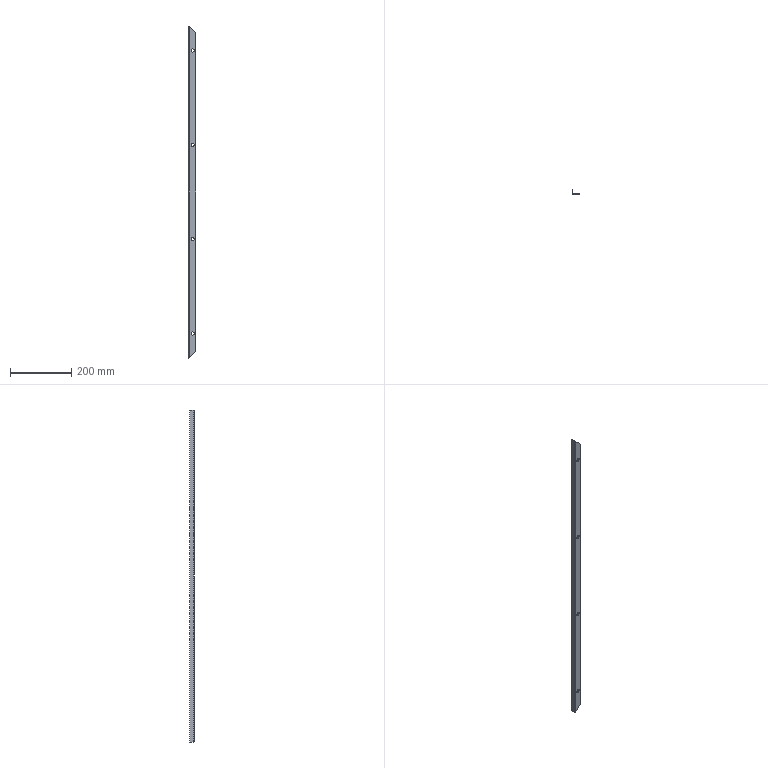Part | STEP file | 750078196 | 1 solid | 22 faces | box 24 x 15 x 1086 mm | volume 75901 mm3 | cylinder 10 | plane 10 | spline 2 | commonest cylinder face diameters 10.5 x8 4 x1 8 x1
STEP:
#1=CARTESIAN_POINT('',(14.,2.,149.083));
#2=VERTEX_POINT('',#1);
#3=CARTESIAN_POINT('',(14.,2.,159.583));
#4=VERTEX_POINT('',#3);
#5=CARTESIAN_POINT('',(14.,2.,154.333));
#6=DIRECTION('',(0.,1.,0.));
#7=DIRECTION('',(0.,0.,-1.));
#8=AXIS2_PLACEMENT_3D('',#5,#6,#7);
#9=CIRCLE('',#8,5.25);
#10=EDGE_CURVE('',#2,#4,#9,.T.);
#11=ORIENTED_EDGE('',*,*,#10,.T.);
#12=CARTESIAN_POINT('',(14.,0.,159.583));
#13=VERTEX_POINT('',#12);
#14=CARTESIAN_POINT('',(14.,1086.369,159.583));
#15=DIRECTION('',(0.,-1.,0.));
#16=VECTOR('',#15,1000.);
#17=LINE('',#14,#16);
#18=EDGE_CURVE('',#4,#13,#17,.T.);
#19=ORIENTED_EDGE('',*,*,#18,.T.);
#20=CARTESIAN_POINT('',(14.,0.,149.083));
#21=VERTEX_POINT('',#20);
#22=CARTESIAN_POINT('',(14.,0.,154.333));
#23=DIRECTION('',(0.,1.,0.));
#24=DIRECTION('',(0.,0.,-1.));
#25=AXIS2_PLACEMENT_3D('',#22,#23,#24);
#26=CIRCLE('',#25,5.25);
#27=EDGE_CURVE('',#21,#13,#26,.T.);
#28=ORIENTED_EDGE('',*,*,#27,.F.);
#29=CARTESIAN_POINT('',(14.,1086.369,149.083));
#30=DIRECTION('',(0.,-1.,0.));
#31=VECTOR('',#30,1000.);
#32=LINE('',#29,#31);
#33=EDGE_CURVE('',#2,#21,#32,.T.);
#34=ORIENTED_EDGE('',*,*,#33,.F.);
#35=EDGE_LOOP('',(#11,#19,#28,#34));
#36=FACE_OUTER_BOUND('',#35,.T.);
#37=CARTESIAN_POINT('',(14.,1086.369,154.333));
#38=DIRECTION('',(0.,-1.,0.));
#39=DIRECTION('',(0.,0.,-1.));
#40=AXIS2_PLACEMENT_3D('',#37,#38,#39);
#41=CYLINDRICAL_SURFACE('',#40,5.25);
#42=ADVANCED_FACE('',(#36),#41,.F.);
#43=CARTESIAN_POINT('',(14.,2.,-468.25));
#44=VERTEX_POINT('',#43);
#45=CARTESIAN_POINT('',(14.,2.,-457.75));
#46=VERTEX_POINT('',#45);
#47=CARTESIAN_POINT('',(14.,2.,-463.));
#48=DIRECTION('',(0.,1.,0.));
#49=DIRECTION('',(0.,0.,-1.));
#50=AXIS2_PLACEMENT_3D('',#47,#48,#49);
#51=CIRCLE('',#50,5.25);
#52=EDGE_CURVE('',#44,#46,#51,.T.);
#53=ORIENTED_EDGE('',*,*,#52,.T.);
#54=CARTESIAN_POINT('',(14.,0.,-457.75));
#55=VERTEX_POINT('',#54);
#56=CARTESIAN_POINT('',(14.,1086.369,-457.75));
#57=DIRECTION('',(0.,-1.,0.));
#58=VECTOR('',#57,1000.);
#59=LINE('',#56,#58);
#60=EDGE_CURVE('',#46,#55,#59,.T.);
#61=ORIENTED_EDGE('',*,*,#60,.T.);
#62=CARTESIAN_POINT('',(14.,0.,-468.25));
#63=VERTEX_POINT('',#62);
#64=CARTESIAN_POINT('',(14.,0.,-463.));
#65=DIRECTION('',(0.,1.,0.));
#66=DIRECTION('',(0.,0.,-1.));
#67=AXIS2_PLACEMENT_3D('',#64,#65,#66);
#68=CIRCLE('',#67,5.25);
#69=EDGE_CURVE('',#63,#55,#68,.T.);
#70=ORIENTED_EDGE('',*,*,#69,.F.);
#71=CARTESIAN_POINT('',(14.,1086.369,-468.25));
#72=DIRECTION('',(0.,-1.,0.));
#73=VECTOR('',#72,1000.);
#74=LINE('',#71,#73);
#75=EDGE_CURVE('',#44,#63,#74,.T.);
#76=ORIENTED_EDGE('',*,*,#75,.F.);
#77=EDGE_LOOP('',(#53,#61,#70,#76));
#78=FACE_OUTER_BOUND('',#77,.T.);
#79=CARTESIAN_POINT('',(14.,1086.369,-463.));
#80=DIRECTION('',(0.,-1.,0.));
#81=DIRECTION('',(0.,0.,-1.));
#82=AXIS2_PLACEMENT_3D('',#79,#80,#81);
#83=CYLINDRICAL_SURFACE('',#82,5.25);
#84=ADVANCED_FACE('',(#78),#83,.F.);
#85=CARTESIAN_POINT('',(14.,2.,-159.583));
#86=VERTEX_POINT('',#85);
#87=CARTESIAN_POINT('',(14.,2.,-149.083));
#88=VERTEX_POINT('',#87);
#89=CARTESIAN_POINT('',(14.,2.,-154.333));
#90=DIRECTION('',(0.,1.,0.));
#91=DIRECTION('',(0.,0.,-1.));
#92=AXIS2_PLACEMENT_3D('',#89,#90,#91);
#93=CIRCLE('',#92,5.25);
#94=EDGE_CURVE('',#86,#88,#93,.T.);
#95=ORIENTED_EDGE('',*,*,#94,.T.);
#96=CARTESIAN_POINT('',(14.,0.,-149.083));
#97=VERTEX_POINT('',#96);
#98=CARTESIAN_POINT('',(14.,1086.369,-149.083));
#99=DIRECTION('',(0.,-1.,0.));
#100=VECTOR('',#99,1000.);
#101=LINE('',#98,#100);
#102=EDGE_CURVE('',#88,#97,#101,.T.);
#103=ORIENTED_EDGE('',*,*,#102,.T.);
#104=CARTESIAN_POINT('',(14.,0.,-159.583));
#105=VERTEX_POINT('',#104);
#106=CARTESIAN_POINT('',(14.,0.,-154.333));
#107=DIRECTION('',(0.,1.,0.));
#108=DIRECTION('',(0.,0.,-1.));
#109=AXIS2_PLACEMENT_3D('',#106,#107,#108);
#110=CIRCLE('',#109,5.25);
#111=EDGE_CURVE('',#105,#97,#110,.T.);
#112=ORIENTED_EDGE('',*,*,#111,.F.);
#113=CARTESIAN_POINT('',(14.,1086.369,-159.583));
#114=DIRECTION('',(0.,-1.,0.));
#115=VECTOR('',#114,1000.);
#116=LINE('',#113,#115);
#117=EDGE_CURVE('',#86,#105,#116,.T.);
#118=ORIENTED_EDGE('',*,*,#117,.F.);
#119=EDGE_LOOP('',(#95,#103,#112,#118));
#120=FACE_OUTER_BOUND('',#119,.T.);
#121=CARTESIAN_POINT('',(14.,1086.369,-154.333));
#122=DIRECTION('',(0.,-1.,0.));
#123=DIRECTION('',(0.,0.,-1.));
#124=AXIS2_PLACEMENT_3D('',#121,#122,#123);
#125=CYLINDRICAL_SURFACE('',#124,5.25);
#126=ADVANCED_FACE('',(#120),#125,.F.);
#127=CARTESIAN_POINT('',(14.,2.,457.75));
#128=VERTEX_POINT('',#127);
#129=CARTESIAN_POINT('',(14.,2.,468.25));
#130=VERTEX_POINT('',#129);
#131=CARTESIAN_POINT('',(14.,2.,463.));
#132=DIRECTION('',(0.,1.,0.));
#133=DIRECTION('',(0.,0.,-1.));
#134=AXIS2_PLACEMENT_3D('',#131,#132,#133);
#135=CIRCLE('',#134,5.25);
#136=EDGE_CURVE('',#128,#130,#135,.T.);
#137=ORIENTED_EDGE('',*,*,#136,.T.);
#138=CARTESIAN_POINT('',(14.,0.,468.25));
#139=VERTEX_POINT('',#138);
#140=CARTESIAN_POINT('',(14.,1086.369,468.25));
#141=DIRECTION('',(0.,-1.,0.));
#142=VECTOR('',#141,1000.);
#143=LINE('',#140,#142);
#144=EDGE_CURVE('',#130,#139,#143,.T.);
#145=ORIENTED_EDGE('',*,*,#144,.T.);
#146=CARTESIAN_POINT('',(14.,0.,457.75));
#147=VERTEX_POINT('',#146);
#148=CARTESIAN_POINT('',(14.,0.,463.));
#149=DIRECTION('',(0.,1.,0.));
#150=DIRECTION('',(0.,0.,-1.));
#151=AXIS2_PLACEMENT_3D('',#148,#149,#150);
#152=CIRCLE('',#151,5.25);
#153=EDGE_CURVE('',#147,#139,#152,.T.);
#154=ORIENTED_EDGE('',*,*,#153,.F.);
#155=CARTESIAN_POINT('',(14.,1086.369,457.75));
#156=DIRECTION('',(0.,-1.,0.));
#157=VECTOR('',#156,1000.);
#158=LINE('',#155,#157);
#159=EDGE_CURVE('',#128,#147,#158,.T.);
#160=ORIENTED_EDGE('',*,*,#159,.F.);
#161=EDGE_LOOP('',(#137,#145,#154,#160));
#162=FACE_OUTER_BOUND('',#161,.T.);
#163=CARTESIAN_POINT('',(14.,1086.369,463.));
#164=DIRECTION('',(0.,-1.,0.));
#165=DIRECTION('',(0.,0.,-1.));
#166=AXIS2_PLACEMENT_3D('',#163,#164,#165);
#167=CYLINDRICAL_SURFACE('',#166,5.25);
#168=ADVANCED_FACE('',(#162),#167,.F.);
#169=CARTESIAN_POINT('',(24.,2.,-521.));
#170=VERTEX_POINT('',#169);
#171=CARTESIAN_POINT('',(24.,2.,521.));
#172=VERTEX_POINT('',#171);
#173=CARTESIAN_POINT('',(24.,2.,543.));
#174=DIRECTION('',(0.,0.,1.));
#175=VECTOR('',#174,1000.);
#176=LINE('',#173,#175);
#177=EDGE_CURVE('',#170,#172,#176,.T.);
#178=ORIENTED_EDGE('',*,*,#177,.F.);
#179=CARTESIAN_POINT('',(4.,2.,-541.));
#180=VERTEX_POINT('',#179);
#181=CARTESIAN_POINT('',(4.,2.,-541.));
#182=DIRECTION('',(0.7071,0.,0.7071));
#183=VECTOR('',#182,1000.);
#184=LINE('',#181,#183);
#185=EDGE_CURVE('',#180,#170,#184,.T.);
#186=ORIENTED_EDGE('',*,*,#185,.F.);
#187=CARTESIAN_POINT('',(4.,2.,541.));
#188=VERTEX_POINT('',#187);
#189=CARTESIAN_POINT('',(4.,2.,543.));
#190=DIRECTION('',(0.,0.,-1.));
#191=VECTOR('',#190,1000.);
#192=LINE('',#189,#191);
#193=EDGE_CURVE('',#188,#180,#192,.T.);
#194=ORIENTED_EDGE('',*,*,#193,.F.);
#195=CARTESIAN_POINT('',(24.,2.,521.));
#196=DIRECTION('',(-0.7071,0.,0.7071));
#197=VECTOR('',#196,1000.);
#198=LINE('',#195,#197);
#199=EDGE_CURVE('',#172,#188,#198,.T.);
#200=ORIENTED_EDGE('',*,*,#199,.F.);
#201=EDGE_LOOP('',(#178,#186,#194,#200));
#202=FACE_OUTER_BOUND('',#201,.T.);
#203=ORIENTED_EDGE('',*,*,#10,.F.);
#204=CARTESIAN_POINT('',(14.,2.,154.333));
#205=DIRECTION('',(0.,1.,0.));
#206=DIRECTION('',(0.,0.,-1.));
#207=AXIS2_PLACEMENT_3D('',#204,#205,#206);
#208=CIRCLE('',#207,5.25);
#209=EDGE_CURVE('',#4,#2,#208,.T.);
#210=ORIENTED_EDGE('',*,*,#209,.F.);
#211=EDGE_LOOP('',(#203,#210));
#212=FACE_BOUND('',#211,.T.);
#213=ORIENTED_EDGE('',*,*,#52,.F.);
#214=CARTESIAN_POINT('',(14.,2.,-463.));
#215=DIRECTION('',(0.,1.,0.));
#216=DIRECTION('',(0.,0.,-1.));
#217=AXIS2_PLACEMENT_3D('',#214,#215,#216);
#218=CIRCLE('',#217,5.25);
#219=EDGE_CURVE('',#46,#44,#218,.T.);
#220=ORIENTED_EDGE('',*,*,#219,.F.);
#221=EDGE_LOOP('',(#213,#220));
#222=FACE_BOUND('',#221,.T.);
#223=ORIENTED_EDGE('',*,*,#94,.F.);
#224=CARTESIAN_POINT('',(14.,2.,-154.333));
#225=DIRECTION('',(0.,1.,0.));
#226=DIRECTION('',(0.,0.,-1.));
#227=AXIS2_PLACEMENT_3D('',#224,#225,#226);
#228=CIRCLE('',#227,5.25);
#229=EDGE_CURVE('',#88,#86,#228,.T.);
#230=ORIENTED_EDGE('',*,*,#229,.F.);
#231=EDGE_LOOP('',(#223,#230));
#232=FACE_BOUND('',#231,.T.);
#233=ORIENTED_EDGE('',*,*,#136,.F.);
#234=CARTESIAN_POINT('',(14.,2.,463.));
#235=DIRECTION('',(0.,1.,0.));
#236=DIRECTION('',(0.,0.,-1.));
#237=AXIS2_PLACEMENT_3D('',#234,#235,#236);
#238=CIRCLE('',#237,5.25);
#239=EDGE_CURVE('',#130,#128,#238,.T.);
#240=ORIENTED_EDGE('',*,*,#239,.F.);
#241=EDGE_LOOP('',(#233,#240));
#242=FACE_BOUND('',#241,.T.);
#243=CARTESIAN_POINT('',(24.,2.,543.));
#244=DIRECTION('',(0.,-1.,0.));
#245=DIRECTION('',(0.,0.,-1.));
#246=AXIS2_PLACEMENT_3D('',#243,#244,#245);
#247=PLANE('',#246);
#248=ADVANCED_FACE('',(#202,#212,#222,#232,#242),#247,.F.);
#249=CARTESIAN_POINT('',(24.,0.,521.));
#250=VERTEX_POINT('',#249);
#251=CARTESIAN_POINT('',(24.,0.,521.));
#252=DIRECTION('',(0.,1.,0.));
#253=VECTOR('',#252,1000.);
#254=LINE('',#251,#253);
#255=EDGE_CURVE('',#250,#172,#254,.T.);
#256=ORIENTED_EDGE('',*,*,#255,.T.);
#257=ORIENTED_EDGE('',*,*,#199,.T.);
#258=CARTESIAN_POINT('',(4.,0.,541.));
#259=VERTEX_POINT('',#258);
#260=CARTESIAN_POINT('',(4.,0.,541.));
#261=DIRECTION('',(0.,-1.,0.));
#262=VECTOR('',#261,1000.);
#263=LINE('',#260,#262);
#264=EDGE_CURVE('',#188,#259,#263,.T.);
#265=ORIENTED_EDGE('',*,*,#264,.T.);
#266=CARTESIAN_POINT('',(13.,0.,532.));
#267=DIRECTION('',(0.7071,0.,-0.7071));
#268=VECTOR('',#267,1000.);
#269=LINE('',#266,#268);
#270=EDGE_CURVE('',#259,#250,#269,.T.);
#271=ORIENTED_EDGE('',*,*,#270,.T.);
#272=EDGE_LOOP('',(#256,#257,#265,#271));
#273=FACE_OUTER_BOUND('',#272,.T.);
#274=CARTESIAN_POINT('',(13.,0.,532.));
#275=DIRECTION('',(0.7071,0.,0.7071));
#276=DIRECTION('',(0.7071,0.,-0.7071));
#277=AXIS2_PLACEMENT_3D('',#274,#275,#276);
#278=PLANE('',#277);
#279=ADVANCED_FACE('',(#273),#278,.T.);
#280=ORIENTED_EDGE('',*,*,#255,.F.);
#281=CARTESIAN_POINT('',(24.,0.,-521.));
#282=VERTEX_POINT('',#281);
#283=CARTESIAN_POINT('',(24.,0.,543.));
#284=DIRECTION('',(0.,0.,1.));
#285=VECTOR('',#284,1000.);
#286=LINE('',#283,#285);
#287=EDGE_CURVE('',#282,#250,#286,.T.);
#288=ORIENTED_EDGE('',*,*,#287,.F.);
#289=CARTESIAN_POINT('',(24.,0.,-521.));
#290=DIRECTION('',(0.,-1.,0.));
#291=VECTOR('',#290,1000.);
#292=LINE('',#289,#291);
#293=EDGE_CURVE('',#170,#282,#292,.T.);
#294=ORIENTED_EDGE('',*,*,#293,.F.);
#295=ORIENTED_EDGE('',*,*,#177,.T.);
#296=EDGE_LOOP('',(#280,#288,#294,#295));
#297=FACE_OUTER_BOUND('',#296,.T.);
#298=CARTESIAN_POINT('',(24.,0.,543.));
#299=DIRECTION('',(-1.,0.,0.));
#300=DIRECTION('',(0.,0.,1.));
#301=AXIS2_PLACEMENT_3D('',#298,#299,#300);
#302=PLANE('',#301);
#303=ADVANCED_FACE('',(#297),#302,.F.);
#304=CARTESIAN_POINT('',(4.,0.,-541.));
#305=VERTEX_POINT('',#304);
#306=CARTESIAN_POINT('',(4.,0.,-541.));
#307=DIRECTION('',(0.,1.,0.));
#308=VECTOR('',#307,1000.);
#309=LINE('',#306,#308);
#310=EDGE_CURVE('',#305,#180,#309,.T.);
#311=ORIENTED_EDGE('',*,*,#310,.T.);
#312=ORIENTED_EDGE('',*,*,#185,.T.);
#313=ORIENTED_EDGE('',*,*,#293,.T.);
#314=CARTESIAN_POINT('',(556.,0.,11.));
#315=DIRECTION('',(-0.7071,0.,-0.7071));
#316=VECTOR('',#315,1000.);
#317=LINE('',#314,#316);
#318=EDGE_CURVE('',#282,#305,#317,.T.);
#319=ORIENTED_EDGE('',*,*,#318,.T.);
#320=EDGE_LOOP('',(#311,#312,#313,#319));
#321=FACE_OUTER_BOUND('',#320,.T.);
#322=CARTESIAN_POINT('',(556.,0.,11.));
#323=DIRECTION('',(0.7071,0.,-0.7071));
#324=DIRECTION('',(-0.7071,0.,-0.7071));
#325=AXIS2_PLACEMENT_3D('',#322,#323,#324);
#326=PLANE('',#325);
#327=ADVANCED_FACE('',(#321),#326,.T.);
#328=ORIENTED_EDGE('',*,*,#193,.T.);
#329=CARTESIAN_POINT('',(2.,4.,-543.));
#330=VERTEX_POINT('',#329);
#331=CARTESIAN_POINT('',(2.,4.,-543.));
#332=CARTESIAN_POINT('',(2.,3.,-543.));
#333=CARTESIAN_POINT('',(2.667,2.,-542.333));
#334=CARTESIAN_POINT('',(4.,2.,-541.));
#335=(BOUNDED_CURVE()B_SPLINE_CURVE(3,(#331,#332,#333,#334),.UNSPECIFIED.,.F.,.F.)B_SPLINE_CURVE_WITH_KNOTS((4,4),(0.,0.003806),.UNSPECIFIED.)CURVE()GEOMETRIC_REPRESENTATION_ITEM()RATIONAL_B_SPLINE_CURVE((1.,0.6667,0.5,0.5))REPRESENTATION_ITEM(''));
#336=EDGE_CURVE('',#330,#180,#335,.T.);
#337=ORIENTED_EDGE('',*,*,#336,.F.);
#338=CARTESIAN_POINT('',(2.,4.,543.));
#339=VERTEX_POINT('',#338);
#340=CARTESIAN_POINT('',(2.,4.,543.));
#341=DIRECTION('',(0.,0.,-1.));
#342=VECTOR('',#341,1000.);
#343=LINE('',#340,#342);
#344=EDGE_CURVE('',#339,#330,#343,.T.);
#345=ORIENTED_EDGE('',*,*,#344,.F.);
#346=CARTESIAN_POINT('',(4.,2.,541.));
#347=CARTESIAN_POINT('',(2.667,2.,542.333));
#348=CARTESIAN_POINT('',(2.,3.,543.));
#349=CARTESIAN_POINT('',(2.,4.,543.));
#350=(BOUNDED_CURVE()B_SPLINE_CURVE(3,(#346,#347,#348,#349),.UNSPECIFIED.,.F.,.F.)B_SPLINE_CURVE_WITH_KNOTS((4,4),(0.,0.003785),.UNSPECIFIED.)CURVE()GEOMETRIC_REPRESENTATION_ITEM()RATIONAL_B_SPLINE_CURVE((0.5,0.5,0.6667,1.))REPRESENTATION_ITEM(''));
#351=EDGE_CURVE('',#188,#339,#350,.T.);
#352=ORIENTED_EDGE('',*,*,#351,.F.);
#353=EDGE_LOOP('',(#328,#337,#345,#352));
#354=FACE_OUTER_BOUND('',#353,.T.);
#355=CARTESIAN_POINT('',(4.,4.,543.));
#356=DIRECTION('',(0.,0.,-1.));
#357=DIRECTION('',(-1.,0.,0.));
#358=AXIS2_PLACEMENT_3D('',#355,#356,#357);
#359=CYLINDRICAL_SURFACE('',#358,2.);
#360=ADVANCED_FACE('',(#354),#359,.F.);
#361=ORIENTED_EDGE('',*,*,#18,.F.);
#362=ORIENTED_EDGE('',*,*,#209,.T.);
#363=ORIENTED_EDGE('',*,*,#33,.T.);
#364=CARTESIAN_POINT('',(14.,0.,154.333));
#365=DIRECTION('',(0.,1.,0.));
#366=DIRECTION('',(0.,0.,-1.));
#367=AXIS2_PLACEMENT_3D('',#364,#365,#366);
#368=CIRCLE('',#367,5.25);
#369=EDGE_CURVE('',#13,#21,#368,.T.);
#370=ORIENTED_EDGE('',*,*,#369,.F.);
#371=EDGE_LOOP('',(#361,#362,#363,#370));
#372=FACE_OUTER_BOUND('',#371,.T.);
#373=CARTESIAN_POINT('',(14.,1086.369,154.333));
#374=DIRECTION('',(0.,-1.,0.));
#375=DIRECTION('',(0.,0.,-1.));
#376=AXIS2_PLACEMENT_3D('',#373,#374,#375);
#377=CYLINDRICAL_SURFACE('',#376,5.25);
#378=ADVANCED_FACE('',(#372),#377,.F.);
#379=ORIENTED_EDGE('',*,*,#60,.F.);
#380=ORIENTED_EDGE('',*,*,#219,.T.);
#381=ORIENTED_EDGE('',*,*,#75,.T.);
#382=CARTESIAN_POINT('',(14.,0.,-463.));
#383=DIRECTION('',(0.,1.,0.));
#384=DIRECTION('',(0.,0.,-1.));
#385=AXIS2_PLACEMENT_3D('',#382,#383,#384);
#386=CIRCLE('',#385,5.25);
#387=EDGE_CURVE('',#55,#63,#386,.T.);
#388=ORIENTED_EDGE('',*,*,#387,.F.);
#389=EDGE_LOOP('',(#379,#380,#381,#388));
#390=FACE_OUTER_BOUND('',#389,.T.);
#391=CARTESIAN_POINT('',(14.,1086.369,-463.));
#392=DIRECTION('',(0.,-1.,0.));
#393=DIRECTION('',(0.,0.,-1.));
#394=AXIS2_PLACEMENT_3D('',#391,#392,#393);
#395=CYLINDRICAL_SURFACE('',#394,5.25);
#396=ADVANCED_FACE('',(#390),#395,.F.);
#397=ORIENTED_EDGE('',*,*,#102,.F.);
#398=ORIENTED_EDGE('',*,*,#229,.T.);
#399=ORIENTED_EDGE('',*,*,#117,.T.);
#400=CARTESIAN_POINT('',(14.,0.,-154.333));
#401=DIRECTION('',(0.,1.,0.));
#402=DIRECTION('',(0.,0.,-1.));
#403=AXIS2_PLACEMENT_3D('',#400,#401,#402);
#404=CIRCLE('',#403,5.25);
#405=EDGE_CURVE('',#97,#105,#404,.T.);
#406=ORIENTED_EDGE('',*,*,#405,.F.);
#407=EDGE_LOOP('',(#397,#398,#399,#406));
#408=FACE_OUTER_BOUND('',#407,.T.);
#409=CARTESIAN_POINT('',(14.,1086.369,-154.333));
#410=DIRECTION('',(0.,-1.,0.));
#411=DIRECTION('',(0.,0.,-1.));
#412=AXIS2_PLACEMENT_3D('',#409,#410,#411);
#413=CYLINDRICAL_SURFACE('',#412,5.25);
#414=ADVANCED_FACE('',(#408),#413,.F.);
#415=ORIENTED_EDGE('',*,*,#144,.F.);
#416=ORIENTED_EDGE('',*,*,#239,.T.);
#417=ORIENTED_EDGE('',*,*,#159,.T.);
#418=CARTESIAN_POINT('',(14.,0.,463.));
#419=DIRECTION('',(0.,1.,0.));
#420=DIRECTION('',(0.,0.,-1.));
#421=AXIS2_PLACEMENT_3D('',#418,#419,#420);
#422=CIRCLE('',#421,5.25);
#423=EDGE_CURVE('',#139,#147,#422,.T.);
#424=ORIENTED_EDGE('',*,*,#423,.F.);
#425=EDGE_LOOP('',(#415,#416,#417,#424));
#426=FACE_OUTER_BOUND('',#425,.T.);
#427=CARTESIAN_POINT('',(14.,1086.369,463.));
#428=DIRECTION('',(0.,-1.,0.));
#429=DIRECTION('',(0.,0.,-1.));
#430=AXIS2_PLACEMENT_3D('',#427,#428,#429);
#431=CYLINDRICAL_SURFACE('',#430,5.25);
#432=ADVANCED_FACE('',(#426),#431,.F.);
#433=CARTESIAN_POINT('',(4.,0.,543.));
#434=DIRECTION('',(0.,0.,-1.));
#435=VECTOR('',#434,1000.);
#436=LINE('',#433,#435);
#437=EDGE_CURVE('',#259,#305,#436,.T.);
#438=ORIENTED_EDGE('',*,*,#437,.T.);
#439=ORIENTED_EDGE('',*,*,#318,.F.);
#440=ORIENTED_EDGE('',*,*,#287,.T.);
#441=ORIENTED_EDGE('',*,*,#270,.F.);
#442=EDGE_LOOP('',(#438,#439,#440,#441));
#443=FACE_OUTER_BOUND('',#442,.T.);
#444=ORIENTED_EDGE('',*,*,#27,.T.);
#445=ORIENTED_EDGE('',*,*,#369,.T.);
#446=EDGE_LOOP('',(#444,#445));
#447=FACE_BOUND('',#446,.T.);
#448=ORIENTED_EDGE('',*,*,#69,.T.);
#449=ORIENTED_EDGE('',*,*,#387,.T.);
#450=EDGE_LOOP('',(#448,#449));
#451=FACE_BOUND('',#450,.T.);
#452=ORIENTED_EDGE('',*,*,#111,.T.);
#453=ORIENTED_EDGE('',*,*,#405,.T.);
#454=EDGE_LOOP('',(#452,#453));
#455=FACE_BOUND('',#454,.T.);
#456=ORIENTED_EDGE('',*,*,#153,.T.);
#457=ORIENTED_EDGE('',*,*,#423,.T.);
#458=EDGE_LOOP('',(#456,#457));
#459=FACE_BOUND('',#458,.T.);
#460=CARTESIAN_POINT('',(24.,0.,543.));
#461=DIRECTION('',(0.,-1.,0.));
#462=DIRECTION('',(0.,0.,-1.));
#463=AXIS2_PLACEMENT_3D('',#460,#461,#462);
#464=PLANE('',#463);
#465=ADVANCED_FACE('',(#443,#447,#451,#455,#459),#464,.T.);
#466=ORIENTED_EDGE('',*,*,#351,.T.);
#467=CARTESIAN_POINT('',(0.,4.,543.));
#468=VERTEX_POINT('',#467);
#469=CARTESIAN_POINT('',(1.,4.,543.));
#470=DIRECTION('',(1.,0.,0.));
#471=VECTOR('',#470,1000.);
#472=LINE('',#469,#471);
#473=EDGE_CURVE('',#468,#339,#472,.T.);
#474=ORIENTED_EDGE('',*,*,#473,.F.);
#475=CARTESIAN_POINT('',(4.,0.,541.));
#476=CARTESIAN_POINT('',(1.333,0.,542.333));
#477=CARTESIAN_POINT('',(0.,2.,543.));
#478=CARTESIAN_POINT('',(0.,4.,543.));
#479=(BOUNDED_CURVE()B_SPLINE_CURVE(3,(#475,#476,#477,#478),.UNSPECIFIED.,.F.,.F.)B_SPLINE_CURVE_WITH_KNOTS((4,4),(0.,0.006641),.UNSPECIFIED.)CURVE()GEOMETRIC_REPRESENTATION_ITEM()RATIONAL_B_SPLINE_CURVE((0.5,0.5,0.6667,1.))REPRESENTATION_ITEM(''));
#480=EDGE_CURVE('',#259,#468,#479,.T.);
#481=ORIENTED_EDGE('',*,*,#480,.F.);
#482=ORIENTED_EDGE('',*,*,#264,.F.);
#483=EDGE_LOOP('',(#466,#474,#481,#482));
#484=FACE_OUTER_BOUND('',#483,.T.);
#485=CARTESIAN_POINT('',(8.,4.,539.));
#486=CARTESIAN_POINT('',(7.333,4.,539.));
#487=CARTESIAN_POINT('',(6.667,4.,539.));
#488=CARTESIAN_POINT('',(6.,4.,539.));
#489=CARTESIAN_POINT('',(8.,-4.,539.));
#490=CARTESIAN_POINT('',(7.333,-2.667,539.));
#491=CARTESIAN_POINT('',(6.667,-1.333,539.));
#492=CARTESIAN_POINT('',(6.,0.,539.));
#493=CARTESIAN_POINT('',(0.,-4.,543.));
#494=CARTESIAN_POINT('',(0.6667,-2.667,543.));
#495=CARTESIAN_POINT('',(1.333,-1.333,543.));
#496=CARTESIAN_POINT('',(2.,0.,543.));
#497=CARTESIAN_POINT('',(0.,4.,543.));
#498=CARTESIAN_POINT('',(0.6667,4.,543.));
#499=CARTESIAN_POINT('',(1.333,4.,543.));
#500=CARTESIAN_POINT('',(2.,4.,543.));
#501=CARTESIAN_POINT('',(0.,12.,543.));
#502=CARTESIAN_POINT('',(0.6667,10.667,543.));
#503=CARTESIAN_POINT('',(1.333,9.333,543.));
#504=CARTESIAN_POINT('',(2.,8.,543.));
#505=CARTESIAN_POINT('',(8.,12.,539.));
#506=CARTESIAN_POINT('',(7.333,10.667,539.));
#507=CARTESIAN_POINT('',(6.667,9.333,539.));
#508=CARTESIAN_POINT('',(6.,8.,539.));
#509=CARTESIAN_POINT('',(8.,4.,539.));
#510=CARTESIAN_POINT('',(7.333,4.,539.));
#511=CARTESIAN_POINT('',(6.667,4.,539.));
#512=CARTESIAN_POINT('',(6.,4.,539.));
#513=(BOUNDED_SURFACE()B_SPLINE_SURFACE(3,3,((#485,#486,#487,#488),(#489,#490,#491,#492),(#493,#494,#495,#496),(#497,#498,#499,#500),(#501,#502,#503,#504),(#505,#506,#507,#508),(#509,#510,#511,#512)),.UNSPECIFIED.,.T.,.F.,.F.)B_SPLINE_SURFACE_WITH_KNOTS((4,3,4),(4,4),(0.,0.5,1.),(0.,1.),.UNSPECIFIED.)GEOMETRIC_REPRESENTATION_ITEM()RATIONAL_B_SPLINE_SURFACE(((1.,1.,1.,1.),(0.3333,0.3333,0.3333,0.3333),(0.3333,0.3333,0.3333,0.3333),(1.,1.,1.,1.),(0.3333,0.3333,0.3333,0.3333),(0.3333,0.3333,0.3333,0.3333),(1.,1.,1.,1.)))REPRESENTATION_ITEM('')SURFACE());
#514=ADVANCED_FACE('',(#484),#513,.F.);
#515=CARTESIAN_POINT('',(0.,4.,-543.));
#516=VERTEX_POINT('',#515);
#517=CARTESIAN_POINT('',(1.,4.,-543.));
#518=DIRECTION('',(-1.,0.,0.));
#519=VECTOR('',#518,1000.);
#520=LINE('',#517,#519);
#521=EDGE_CURVE('',#330,#516,#520,.T.);
#522=ORIENTED_EDGE('',*,*,#521,.F.);
#523=ORIENTED_EDGE('',*,*,#336,.T.);
#524=ORIENTED_EDGE('',*,*,#310,.F.);
#525=CARTESIAN_POINT('',(0.,4.,-543.));
#526=CARTESIAN_POINT('',(0.,2.,-543.));
#527=CARTESIAN_POINT('',(1.333,0.,-542.333));
#528=CARTESIAN_POINT('',(4.,0.,-541.));
#529=(BOUNDED_CURVE()B_SPLINE_CURVE(3,(#525,#526,#527,#528),.UNSPECIFIED.,.F.,.F.)B_SPLINE_CURVE_WITH_KNOTS((4,4),(0.,0.006627),.UNSPECIFIED.)CURVE()GEOMETRIC_REPRESENTATION_ITEM()RATIONAL_B_SPLINE_CURVE((1.,0.6667,0.5,0.5))REPRESENTATION_ITEM(''));
#530=EDGE_CURVE('',#516,#305,#529,.T.);
#531=ORIENTED_EDGE('',*,*,#530,.F.);
#532=EDGE_LOOP('',(#522,#523,#524,#531));
#533=FACE_OUTER_BOUND('',#532,.T.);
#534=CARTESIAN_POINT('',(0.,4.,-543.));
#535=CARTESIAN_POINT('',(0.6667,4.,-543.));
#536=CARTESIAN_POINT('',(1.333,4.,-543.));
#537=CARTESIAN_POINT('',(2.,4.,-543.));
#538=CARTESIAN_POINT('',(0.,-4.,-543.));
#539=CARTESIAN_POINT('',(0.6667,-2.667,-543.));
#540=CARTESIAN_POINT('',(1.333,-1.333,-543.));
#541=CARTESIAN_POINT('',(2.,0.,-543.));
#542=CARTESIAN_POINT('',(8.,-4.,-539.));
#543=CARTESIAN_POINT('',(7.333,-2.667,-539.));
#544=CARTESIAN_POINT('',(6.667,-1.333,-539.));
#545=CARTESIAN_POINT('',(6.,0.,-539.));
#546=CARTESIAN_POINT('',(8.,4.,-539.));
#547=CARTESIAN_POINT('',(7.333,4.,-539.));
#548=CARTESIAN_POINT('',(6.667,4.,-539.));
#549=CARTESIAN_POINT('',(6.,4.,-539.));
#550=CARTESIAN_POINT('',(8.,12.,-539.));
#551=CARTESIAN_POINT('',(7.333,10.667,-539.));
#552=CARTESIAN_POINT('',(6.667,9.333,-539.));
#553=CARTESIAN_POINT('',(6.,8.,-539.));
#554=CARTESIAN_POINT('',(0.,12.,-543.));
#555=CARTESIAN_POINT('',(0.6667,10.667,-543.));
#556=CARTESIAN_POINT('',(1.333,9.333,-543.));
#557=CARTESIAN_POINT('',(2.,8.,-543.));
#558=CARTESIAN_POINT('',(0.,4.,-543.));
#559=CARTESIAN_POINT('',(0.6667,4.,-543.));
#560=CARTESIAN_POINT('',(1.333,4.,-543.));
#561=CARTESIAN_POINT('',(2.,4.,-543.));
#562=(BOUNDED_SURFACE()B_SPLINE_SURFACE(3,3,((#534,#535,#536,#537),(#538,#539,#540,#541),(#542,#543,#544,#545),(#546,#547,#548,#549),(#550,#551,#552,#553),(#554,#555,#556,#557),(#558,#559,#560,#561)),.UNSPECIFIED.,.T.,.F.,.F.)B_SPLINE_SURFACE_WITH_KNOTS((4,3,4),(4,4),(0.,0.5,1.),(0.,1.),.UNSPECIFIED.)GEOMETRIC_REPRESENTATION_ITEM()RATIONAL_B_SPLINE_SURFACE(((1.,1.,1.,1.),(0.3333,0.3333,0.3333,0.3333),(0.3333,0.3333,0.3333,0.3333),(1.,1.,1.,1.),(0.3333,0.3333,0.3333,0.3333),(0.3333,0.3333,0.3333,0.3333),(1.,1.,1.,1.)))REPRESENTATION_ITEM('')SURFACE());
#563=ADVANCED_FACE('',(#533),#562,.F.);
#564=CARTESIAN_POINT('',(2.,15.,543.));
#565=VERTEX_POINT('',#564);
#566=CARTESIAN_POINT('',(2.,15.,-543.));
#567=VERTEX_POINT('',#566);
#568=CARTESIAN_POINT('',(2.,15.,543.));
#569=DIRECTION('',(0.,0.,-1.));
#570=VECTOR('',#569,1000.);
#571=LINE('',#568,#570);
#572=EDGE_CURVE('',#565,#567,#571,.T.);
#573=ORIENTED_EDGE('',*,*,#572,.F.);
#574=CARTESIAN_POINT('',(2.,0.,543.));
#575=DIRECTION('',(0.,1.,0.));
#576=VECTOR('',#575,1000.);
#577=LINE('',#574,#576);
#578=EDGE_CURVE('',#339,#565,#577,.T.);
#579=ORIENTED_EDGE('',*,*,#578,.F.);
#580=ORIENTED_EDGE('',*,*,#344,.T.);
#581=CARTESIAN_POINT('',(2.,0.,-543.));
#582=DIRECTION('',(0.,-1.,0.));
#583=VECTOR('',#582,1000.);
#584=LINE('',#581,#583);
#585=EDGE_CURVE('',#567,#330,#584,.T.);
#586=ORIENTED_EDGE('',*,*,#585,.F.);
#587=EDGE_LOOP('',(#573,#579,#580,#586));
#588=FACE_OUTER_BOUND('',#587,.T.);
#589=CARTESIAN_POINT('',(2.,0.,543.));
#590=DIRECTION('',(-1.,0.,0.));
#591=DIRECTION('',(0.,-1.,0.));
#592=AXIS2_PLACEMENT_3D('',#589,#590,#591);
#593=PLANE('',#592);
#594=ADVANCED_FACE('',(#588),#593,.F.);
#595=CARTESIAN_POINT('',(0.,4.,543.));
#596=DIRECTION('',(0.,0.,-1.));
#597=VECTOR('',#596,1000.);
#598=LINE('',#595,#597);
#599=EDGE_CURVE('',#468,#516,#598,.T.);
#600=ORIENTED_EDGE('',*,*,#599,.T.);
#601=ORIENTED_EDGE('',*,*,#530,.T.);
#602=ORIENTED_EDGE('',*,*,#437,.F.);
#603=ORIENTED_EDGE('',*,*,#480,.T.);
#604=EDGE_LOOP('',(#600,#601,#602,#603));
#605=FACE_OUTER_BOUND('',#604,.T.);
#606=CARTESIAN_POINT('',(4.,4.,543.));
#607=DIRECTION('',(0.,0.,-1.));
#608=DIRECTION('',(-1.,0.,0.));
#609=AXIS2_PLACEMENT_3D('',#606,#607,#608);
#610=CYLINDRICAL_SURFACE('',#609,4.);
#611=ADVANCED_FACE('',(#605),#610,.T.);
#612=ORIENTED_EDGE('',*,*,#578,.T.);
#613=CARTESIAN_POINT('',(0.,15.,543.));
#614=VERTEX_POINT('',#613);
#615=CARTESIAN_POINT('',(0.,15.,543.));
#616=DIRECTION('',(-1.,0.,0.));
#617=VECTOR('',#616,1000.);
#618=LINE('',#615,#617);
#619=EDGE_CURVE('',#565,#614,#618,.T.);
#620=ORIENTED_EDGE('',*,*,#619,.T.);
#621=CARTESIAN_POINT('',(0.,0.,543.));
#622=DIRECTION('',(0.,-1.,0.));
#623=VECTOR('',#622,1000.);
#624=LINE('',#621,#623);
#625=EDGE_CURVE('',#614,#468,#624,.T.);
#626=ORIENTED_EDGE('',*,*,#625,.T.);
#627=ORIENTED_EDGE('',*,*,#473,.T.);
#628=EDGE_LOOP('',(#612,#620,#626,#627));
#629=FACE_OUTER_BOUND('',#628,.T.);
#630=CARTESIAN_POINT('',(0.,0.,543.));
#631=DIRECTION('',(0.,0.,1.));
#632=DIRECTION('',(1.,0.,0.));
#633=AXIS2_PLACEMENT_3D('',#630,#631,#632);
#634=PLANE('',#633);
#635=ADVANCED_FACE('',(#629),#634,.T.);
#636=CARTESIAN_POINT('',(0.,15.,-543.));
#637=VERTEX_POINT('',#636);
#638=CARTESIAN_POINT('',(0.,0.,-543.));
#639=DIRECTION('',(0.,-1.,0.));
#640=VECTOR('',#639,1000.);
#641=LINE('',#638,#640);
#642=EDGE_CURVE('',#637,#516,#641,.T.);
#643=ORIENTED_EDGE('',*,*,#642,.F.);
#644=CARTESIAN_POINT('',(24.,15.,-543.));
#645=DIRECTION('',(-1.,0.,0.));
#646=VECTOR('',#645,1000.);
#647=LINE('',#644,#646);
#648=EDGE_CURVE('',#567,#637,#647,.T.);
#649=ORIENTED_EDGE('',*,*,#648,.F.);
#650=ORIENTED_EDGE('',*,*,#585,.T.);
#651=ORIENTED_EDGE('',*,*,#521,.T.);
#652=EDGE_LOOP('',(#643,#649,#650,#651));
#653=FACE_OUTER_BOUND('',#652,.T.);
#654=CARTESIAN_POINT('',(24.,0.,-543.));
#655=DIRECTION('',(0.,0.,1.));
#656=DIRECTION('',(1.,0.,0.));
#657=AXIS2_PLACEMENT_3D('',#654,#655,#656);
#658=PLANE('',#657);
#659=ADVANCED_FACE('',(#653),#658,.F.);
#660=ORIENTED_EDGE('',*,*,#648,.T.);
#661=CARTESIAN_POINT('',(0.,15.,543.));
#662=DIRECTION('',(0.,0.,1.));
#663=VECTOR('',#662,1000.);
#664=LINE('',#661,#663);
#665=EDGE_CURVE('',#637,#614,#664,.T.);
#666=ORIENTED_EDGE('',*,*,#665,.T.);
#667=ORIENTED_EDGE('',*,*,#619,.F.);
#668=ORIENTED_EDGE('',*,*,#572,.T.);
#669=EDGE_LOOP('',(#660,#666,#667,#668));
#670=FACE_OUTER_BOUND('',#669,.T.);
#671=CARTESIAN_POINT('',(0.,15.,543.));
#672=DIRECTION('',(0.,1.,0.));
#673=DIRECTION('',(-1.,0.,0.));
#674=AXIS2_PLACEMENT_3D('',#671,#672,#673);
#675=PLANE('',#674);
#676=ADVANCED_FACE('',(#670),#675,.T.);
#677=ORIENTED_EDGE('',*,*,#625,.F.);
#678=ORIENTED_EDGE('',*,*,#665,.F.);
#679=ORIENTED_EDGE('',*,*,#642,.T.);
#680=ORIENTED_EDGE('',*,*,#599,.F.);
#681=EDGE_LOOP('',(#677,#678,#679,#680));
#682=FACE_OUTER_BOUND('',#681,.T.);
#683=CARTESIAN_POINT('',(0.,0.,543.));
#684=DIRECTION('',(-1.,0.,0.));
#685=DIRECTION('',(0.,-1.,0.));
#686=AXIS2_PLACEMENT_3D('',#683,#684,#685);
#687=PLANE('',#686);
#688=ADVANCED_FACE('',(#682),#687,.T.);
#689=CLOSED_SHELL('',(#42,#84,#126,#168,#248,#279,#303,#327,#360,#378,#396,#414,#432,#465,#514,#563,#594,#611,#635,#659,#676,#688));
#690=MANIFOLD_SOLID_BREP('',#689);
#691=CARTESIAN_POINT('',(0.,0.,0.));
#692=DIRECTION('',(0.,0.,1.));
#693=DIRECTION('',(1.,0.,0.));
#694=AXIS2_PLACEMENT_3D('',#691,#692,#693);
#695=(LENGTH_UNIT()NAMED_UNIT(*)SI_UNIT(.MILLI.,.METRE.));
#696=UNCERTAINTY_MEASURE_WITH_UNIT(LENGTH_MEASURE(0.00001),#695,'','');
#697=(NAMED_UNIT(*)PLANE_ANGLE_UNIT()SI_UNIT($,.RADIAN.));
#698=(NAMED_UNIT(*)SI_UNIT($,.STERADIAN.)SOLID_ANGLE_UNIT());
#699=(GEOMETRIC_REPRESENTATION_CONTEXT(3)GLOBAL_UNCERTAINTY_ASSIGNED_CONTEXT((#696))GLOBAL_UNIT_ASSIGNED_CONTEXT((#695,#697,#698))REPRESENTATION_CONTEXT('',''));
#700=ADVANCED_BREP_SHAPE_REPRESENTATION('',(#690,#694),#699);